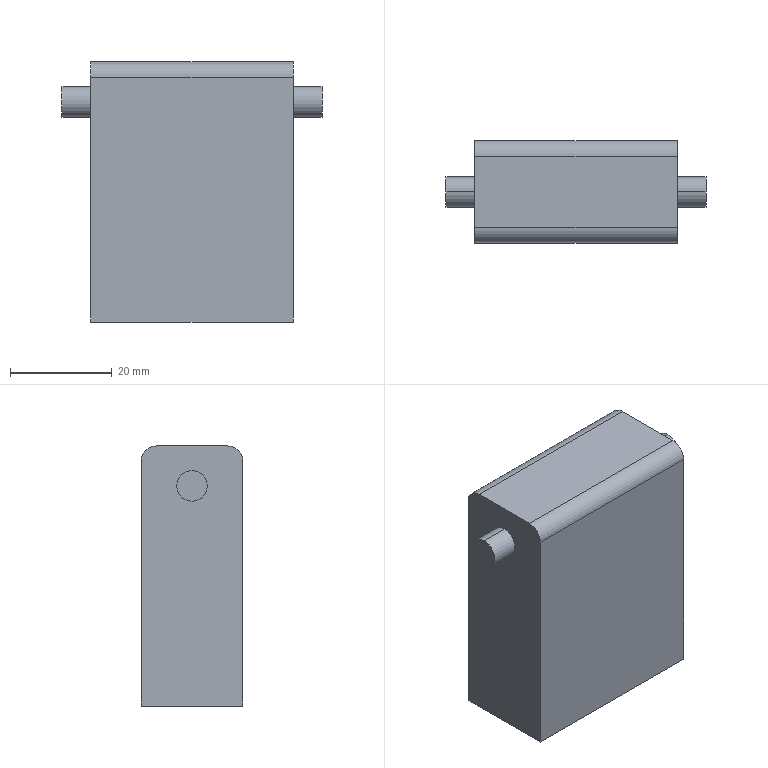Part | SolidWorks | features 3DProfileFeature 1, Extrusion 1, Fillet 1, HoleWzd 1, ICE 1 | 1 solid | 26 faces | box 51 x 20 x 51 mm | volume 40645 mm3 | cylinder 12 | plane 8 | cone 6 | commonest cylinder face diameters 2.5 x6 6 x6
STEP:
#1=CARTESIAN_POINT('',(13.75,0.,7.5));
#2=VERTEX_POINT('',#1);
#3=CARTESIAN_POINT('',(11.25,0.,7.5));
#4=VERTEX_POINT('',#3);
#5=CARTESIAN_POINT('',(12.5,0.,7.5));
#6=DIRECTION('',(0.,0.,-1.));
#7=DIRECTION('',(-1.,0.,0.));
#8=AXIS2_PLACEMENT_3D('',#5,#6,#7);
#9=CIRCLE('',#8,1.25);
#10=EDGE_CURVE('',#2,#4,#9,.T.);
#11=ORIENTED_EDGE('',*,*,#10,.F.);
#12=CARTESIAN_POINT('',(13.75,0.,0.));
#13=VERTEX_POINT('',#12);
#14=CARTESIAN_POINT('',(13.75,0.,0.));
#15=DIRECTION('',(0.,0.,-1.));
#16=VECTOR('',#15,1000.);
#17=LINE('',#14,#16);
#18=EDGE_CURVE('',#2,#13,#17,.T.);
#19=ORIENTED_EDGE('',*,*,#18,.T.);
#20=CARTESIAN_POINT('',(11.25,0.,0.));
#21=VERTEX_POINT('',#20);
#22=CARTESIAN_POINT('',(12.5,0.,0.));
#23=DIRECTION('',(0.,0.,-1.));
#24=DIRECTION('',(-1.,0.,0.));
#25=AXIS2_PLACEMENT_3D('',#22,#23,#24);
#26=CIRCLE('',#25,1.25);
#27=EDGE_CURVE('',#13,#21,#26,.T.);
#28=ORIENTED_EDGE('',*,*,#27,.T.);
#29=CARTESIAN_POINT('',(11.25,0.,0.));
#30=DIRECTION('',(0.,0.,-1.));
#31=VECTOR('',#30,1000.);
#32=LINE('',#29,#31);
#33=EDGE_CURVE('',#4,#21,#32,.T.);
#34=ORIENTED_EDGE('',*,*,#33,.F.);
#35=EDGE_LOOP('',(#11,#19,#28,#34));
#36=FACE_OUTER_BOUND('',#35,.T.);
#37=CARTESIAN_POINT('',(12.5,0.,0.));
#38=DIRECTION('',(0.,0.,-1.));
#39=DIRECTION('',(-1.,0.,0.));
#40=AXIS2_PLACEMENT_3D('',#37,#38,#39);
#41=CYLINDRICAL_SURFACE('',#40,1.25);
#42=ADVANCED_FACE('',(#36),#41,.F.);
#43=CARTESIAN_POINT('',(12.5,0.,8.251));
#44=VERTEX_POINT('',#43);
#45=CARTESIAN_POINT('',(11.25,0.,7.5));
#46=DIRECTION('',(-0.8572,0.,-0.515));
#47=VECTOR('',#46,1000.);
#48=LINE('',#45,#47);
#49=EDGE_CURVE('',#44,#4,#48,.T.);
#50=ORIENTED_EDGE('',*,*,#49,.F.);
#51=CARTESIAN_POINT('',(13.75,0.,7.5));
#52=DIRECTION('',(0.8572,0.,-0.515));
#53=VECTOR('',#52,1000.);
#54=LINE('',#51,#53);
#55=EDGE_CURVE('',#44,#2,#54,.T.);
#56=ORIENTED_EDGE('',*,*,#55,.T.);
#57=ORIENTED_EDGE('',*,*,#10,.T.);
#58=EDGE_LOOP('',(#50,#56,#57));
#59=FACE_OUTER_BOUND('',#58,.T.);
#60=CARTESIAN_POINT('',(12.5,0.,7.5));
#61=DIRECTION('',(0.,0.,-1.));
#62=DIRECTION('',(-1.,0.,0.));
#63=AXIS2_PLACEMENT_3D('',#60,#61,#62);
#64=CONICAL_SURFACE('',#63,1.25,1.03);
#65=ADVANCED_FACE('',(#59),#64,.F.);
#66=CARTESIAN_POINT('',(-11.25,0.,7.5));
#67=VERTEX_POINT('',#66);
#68=CARTESIAN_POINT('',(-13.75,0.,7.5));
#69=VERTEX_POINT('',#68);
#70=CARTESIAN_POINT('',(-12.5,0.,7.5));
#71=DIRECTION('',(0.,0.,-1.));
#72=DIRECTION('',(-1.,0.,0.));
#73=AXIS2_PLACEMENT_3D('',#70,#71,#72);
#74=CIRCLE('',#73,1.25);
#75=EDGE_CURVE('',#67,#69,#74,.T.);
#76=ORIENTED_EDGE('',*,*,#75,.F.);
#77=CARTESIAN_POINT('',(-11.25,0.,0.));
#78=VERTEX_POINT('',#77);
#79=CARTESIAN_POINT('',(-11.25,0.,0.));
#80=DIRECTION('',(0.,0.,-1.));
#81=VECTOR('',#80,1000.);
#82=LINE('',#79,#81);
#83=EDGE_CURVE('',#67,#78,#82,.T.);
#84=ORIENTED_EDGE('',*,*,#83,.T.);
#85=CARTESIAN_POINT('',(-13.75,0.,0.));
#86=VERTEX_POINT('',#85);
#87=CARTESIAN_POINT('',(-12.5,0.,0.));
#88=DIRECTION('',(0.,0.,-1.));
#89=DIRECTION('',(-1.,0.,0.));
#90=AXIS2_PLACEMENT_3D('',#87,#88,#89);
#91=CIRCLE('',#90,1.25);
#92=EDGE_CURVE('',#78,#86,#91,.T.);
#93=ORIENTED_EDGE('',*,*,#92,.T.);
#94=CARTESIAN_POINT('',(-13.75,0.,0.));
#95=DIRECTION('',(0.,0.,-1.));
#96=VECTOR('',#95,1000.);
#97=LINE('',#94,#96);
#98=EDGE_CURVE('',#69,#86,#97,.T.);
#99=ORIENTED_EDGE('',*,*,#98,.F.);
#100=EDGE_LOOP('',(#76,#84,#93,#99));
#101=FACE_OUTER_BOUND('',#100,.T.);
#102=CARTESIAN_POINT('',(-12.5,0.,0.));
#103=DIRECTION('',(0.,0.,-1.));
#104=DIRECTION('',(-1.,0.,0.));
#105=AXIS2_PLACEMENT_3D('',#102,#103,#104);
#106=CYLINDRICAL_SURFACE('',#105,1.25);
#107=ADVANCED_FACE('',(#101),#106,.F.);
#108=CARTESIAN_POINT('',(-12.5,0.,8.251));
#109=VERTEX_POINT('',#108);
#110=CARTESIAN_POINT('',(-13.75,0.,7.5));
#111=DIRECTION('',(-0.8572,0.,-0.515));
#112=VECTOR('',#111,1000.);
#113=LINE('',#110,#112);
#114=EDGE_CURVE('',#109,#69,#113,.T.);
#115=ORIENTED_EDGE('',*,*,#114,.F.);
#116=CARTESIAN_POINT('',(-11.25,0.,7.5));
#117=DIRECTION('',(0.8572,0.,-0.515));
#118=VECTOR('',#117,1000.);
#119=LINE('',#116,#118);
#120=EDGE_CURVE('',#109,#67,#119,.T.);
#121=ORIENTED_EDGE('',*,*,#120,.T.);
#122=ORIENTED_EDGE('',*,*,#75,.T.);
#123=EDGE_LOOP('',(#115,#121,#122));
#124=FACE_OUTER_BOUND('',#123,.T.);
#125=CARTESIAN_POINT('',(-12.5,0.,7.5));
#126=DIRECTION('',(0.,0.,-1.));
#127=DIRECTION('',(-1.,0.,0.));
#128=AXIS2_PLACEMENT_3D('',#125,#126,#127);
#129=CONICAL_SURFACE('',#128,1.25,1.03);
#130=ADVANCED_FACE('',(#124),#129,.F.);
#131=CARTESIAN_POINT('',(1.129,0.,7.5));
#132=VERTEX_POINT('',#131);
#133=CARTESIAN_POINT('',(-1.371,0.,7.5));
#134=VERTEX_POINT('',#133);
#135=CARTESIAN_POINT('',(-0.1209,0.,7.5));
#136=DIRECTION('',(0.,0.,-1.));
#137=DIRECTION('',(-1.,0.,0.));
#138=AXIS2_PLACEMENT_3D('',#135,#136,#137);
#139=CIRCLE('',#138,1.25);
#140=EDGE_CURVE('',#132,#134,#139,.T.);
#141=ORIENTED_EDGE('',*,*,#140,.F.);
#142=CARTESIAN_POINT('',(1.129,0.,0.));
#143=VERTEX_POINT('',#142);
#144=CARTESIAN_POINT('',(1.129,0.,0.));
#145=DIRECTION('',(0.,0.,-1.));
#146=VECTOR('',#145,1000.);
#147=LINE('',#144,#146);
#148=EDGE_CURVE('',#132,#143,#147,.T.);
#149=ORIENTED_EDGE('',*,*,#148,.T.);
#150=CARTESIAN_POINT('',(-1.371,0.,0.));
#151=VERTEX_POINT('',#150);
#152=CARTESIAN_POINT('',(-0.1209,0.,0.));
#153=DIRECTION('',(0.,0.,-1.));
#154=DIRECTION('',(-1.,0.,0.));
#155=AXIS2_PLACEMENT_3D('',#152,#153,#154);
#156=CIRCLE('',#155,1.25);
#157=EDGE_CURVE('',#143,#151,#156,.T.);
#158=ORIENTED_EDGE('',*,*,#157,.T.);
#159=CARTESIAN_POINT('',(-1.371,0.,0.));
#160=DIRECTION('',(0.,0.,-1.));
#161=VECTOR('',#160,1000.);
#162=LINE('',#159,#161);
#163=EDGE_CURVE('',#134,#151,#162,.T.);
#164=ORIENTED_EDGE('',*,*,#163,.F.);
#165=EDGE_LOOP('',(#141,#149,#158,#164));
#166=FACE_OUTER_BOUND('',#165,.T.);
#167=CARTESIAN_POINT('',(-0.1209,0.,0.));
#168=DIRECTION('',(0.,0.,-1.));
#169=DIRECTION('',(-1.,0.,0.));
#170=AXIS2_PLACEMENT_3D('',#167,#168,#169);
#171=CYLINDRICAL_SURFACE('',#170,1.25);
#172=ADVANCED_FACE('',(#166),#171,.F.);
#173=CARTESIAN_POINT('',(-0.1209,0.,8.251));
#174=VERTEX_POINT('',#173);
#175=CARTESIAN_POINT('',(-1.371,0.,7.5));
#176=DIRECTION('',(-0.8572,0.,-0.515));
#177=VECTOR('',#176,1000.);
#178=LINE('',#175,#177);
#179=EDGE_CURVE('',#174,#134,#178,.T.);
#180=ORIENTED_EDGE('',*,*,#179,.F.);
#181=CARTESIAN_POINT('',(1.129,0.,7.5));
#182=DIRECTION('',(0.8572,0.,-0.515));
#183=VECTOR('',#182,1000.);
#184=LINE('',#181,#183);
#185=EDGE_CURVE('',#174,#132,#184,.T.);
#186=ORIENTED_EDGE('',*,*,#185,.T.);
#187=ORIENTED_EDGE('',*,*,#140,.T.);
#188=EDGE_LOOP('',(#180,#186,#187));
#189=FACE_OUTER_BOUND('',#188,.T.);
#190=CARTESIAN_POINT('',(-0.1209,0.,7.5));
#191=DIRECTION('',(0.,0.,-1.));
#192=DIRECTION('',(-1.,0.,0.));
#193=AXIS2_PLACEMENT_3D('',#190,#191,#192);
#194=CONICAL_SURFACE('',#193,1.25,1.03);
#195=ADVANCED_FACE('',(#189),#194,.F.);
#196=CARTESIAN_POINT('',(25.5,0.,40.174));
#197=VERTEX_POINT('',#196);
#198=CARTESIAN_POINT('',(25.5,0.,46.174));
#199=VERTEX_POINT('',#198);
#200=CARTESIAN_POINT('',(25.5,0.,43.174));
#201=DIRECTION('',(1.,0.,0.));
#202=DIRECTION('',(0.,0.,-1.));
#203=AXIS2_PLACEMENT_3D('',#200,#201,#202);
#204=CIRCLE('',#203,3.);
#205=EDGE_CURVE('',#197,#199,#204,.T.);
#206=ORIENTED_EDGE('',*,*,#205,.F.);
#207=CARTESIAN_POINT('',(19.9,0.,40.174));
#208=VERTEX_POINT('',#207);
#209=CARTESIAN_POINT('',(25.5,0.,40.174));
#210=DIRECTION('',(-1.,0.,0.));
#211=VECTOR('',#210,1000.);
#212=LINE('',#209,#211);
#213=EDGE_CURVE('',#197,#208,#212,.T.);
#214=ORIENTED_EDGE('',*,*,#213,.T.);
#215=CARTESIAN_POINT('',(19.9,0.,46.174));
#216=VERTEX_POINT('',#215);
#217=CARTESIAN_POINT('',(19.9,0.,43.174));
#218=DIRECTION('',(1.,0.,0.));
#219=DIRECTION('',(0.,-1.,0.));
#220=AXIS2_PLACEMENT_3D('',#217,#218,#219);
#221=CIRCLE('',#220,3.);
#222=EDGE_CURVE('',#208,#216,#221,.T.);
#223=ORIENTED_EDGE('',*,*,#222,.T.);
#224=CARTESIAN_POINT('',(25.5,0.,46.174));
#225=DIRECTION('',(-1.,0.,0.));
#226=VECTOR('',#225,1000.);
#227=LINE('',#224,#226);
#228=EDGE_CURVE('',#199,#216,#227,.T.);
#229=ORIENTED_EDGE('',*,*,#228,.F.);
#230=EDGE_LOOP('',(#206,#214,#223,#229));
#231=FACE_OUTER_BOUND('',#230,.T.);
#232=CARTESIAN_POINT('',(25.5,0.,43.174));
#233=DIRECTION('',(-1.,0.,0.));
#234=DIRECTION('',(0.,0.,1.));
#235=AXIS2_PLACEMENT_3D('',#232,#233,#234);
#236=CYLINDRICAL_SURFACE('',#235,3.);
#237=ADVANCED_FACE('',(#231),#236,.T.);
#238=CARTESIAN_POINT('',(-19.9,0.,46.174));
#239=VERTEX_POINT('',#238);
#240=CARTESIAN_POINT('',(-19.9,0.,40.174));
#241=VERTEX_POINT('',#240);
#242=CARTESIAN_POINT('',(-19.9,0.,43.174));
#243=DIRECTION('',(-1.,0.,0.));
#244=DIRECTION('',(0.,1.,0.));
#245=AXIS2_PLACEMENT_3D('',#242,#243,#244);
#246=CIRCLE('',#245,3.);
#247=EDGE_CURVE('',#239,#241,#246,.T.);
#248=ORIENTED_EDGE('',*,*,#247,.T.);
#249=CARTESIAN_POINT('',(-25.5,0.,40.174));
#250=VERTEX_POINT('',#249);
#251=CARTESIAN_POINT('',(25.5,0.,40.174));
#252=DIRECTION('',(-1.,0.,0.));
#253=VECTOR('',#252,1000.);
#254=LINE('',#251,#253);
#255=EDGE_CURVE('',#241,#250,#254,.T.);
#256=ORIENTED_EDGE('',*,*,#255,.T.);
#257=CARTESIAN_POINT('',(-25.5,0.,46.174));
#258=VERTEX_POINT('',#257);
#259=CARTESIAN_POINT('',(-25.5,0.,43.174));
#260=DIRECTION('',(1.,0.,0.));
#261=DIRECTION('',(0.,0.,-1.));
#262=AXIS2_PLACEMENT_3D('',#259,#260,#261);
#263=CIRCLE('',#262,3.);
#264=EDGE_CURVE('',#250,#258,#263,.T.);
#265=ORIENTED_EDGE('',*,*,#264,.T.);
#266=CARTESIAN_POINT('',(25.5,0.,46.174));
#267=DIRECTION('',(-1.,0.,0.));
#268=VECTOR('',#267,1000.);
#269=LINE('',#266,#268);
#270=EDGE_CURVE('',#239,#258,#269,.T.);
#271=ORIENTED_EDGE('',*,*,#270,.F.);
#272=EDGE_LOOP('',(#248,#256,#265,#271));
#273=FACE_OUTER_BOUND('',#272,.T.);
#274=CARTESIAN_POINT('',(25.5,0.,43.174));
#275=DIRECTION('',(-1.,0.,0.));
#276=DIRECTION('',(0.,0.,1.));
#277=AXIS2_PLACEMENT_3D('',#274,#275,#276);
#278=CYLINDRICAL_SURFACE('',#277,3.);
#279=ADVANCED_FACE('',(#273),#278,.T.);
#280=CARTESIAN_POINT('',(19.9,0.,43.174));
#281=DIRECTION('',(1.,0.,0.));
#282=DIRECTION('',(0.,-1.,0.));
#283=AXIS2_PLACEMENT_3D('',#280,#281,#282);
#284=CIRCLE('',#283,3.);
#285=EDGE_CURVE('',#216,#208,#284,.T.);
#286=ORIENTED_EDGE('',*,*,#285,.F.);
#287=ORIENTED_EDGE('',*,*,#222,.F.);
#288=EDGE_LOOP('',(#286,#287));
#289=FACE_BOUND('',#288,.T.);
#290=CARTESIAN_POINT('',(19.9,-7.,51.));
#291=VERTEX_POINT('',#290);
#292=CARTESIAN_POINT('',(19.9,7.,51.));
#293=VERTEX_POINT('',#292);
#294=CARTESIAN_POINT('',(19.9,10.,51.));
#295=DIRECTION('',(0.,1.,0.));
#296=VECTOR('',#295,1000.);
#297=LINE('',#294,#296);
#298=EDGE_CURVE('',#291,#293,#297,.T.);
#299=ORIENTED_EDGE('',*,*,#298,.F.);
#300=CARTESIAN_POINT('',(19.9,-10.,48.));
#301=VERTEX_POINT('',#300);
#302=CARTESIAN_POINT('',(19.9,-7.,48.));
#303=DIRECTION('',(1.,0.,0.));
#304=DIRECTION('',(0.,-1.,0.));
#305=AXIS2_PLACEMENT_3D('',#302,#303,#304);
#306=CIRCLE('',#305,3.);
#307=EDGE_CURVE('',#291,#301,#306,.T.);
#308=ORIENTED_EDGE('',*,*,#307,.T.);
#309=CARTESIAN_POINT('',(19.9,-10.,0.));
#310=VERTEX_POINT('',#309);
#311=CARTESIAN_POINT('',(19.9,-10.,51.));
#312=DIRECTION('',(0.,0.,-1.));
#313=VECTOR('',#312,1000.);
#314=LINE('',#311,#313);
#315=EDGE_CURVE('',#301,#310,#314,.T.);
#316=ORIENTED_EDGE('',*,*,#315,.T.);
#317=CARTESIAN_POINT('',(19.9,10.,0.));
#318=VERTEX_POINT('',#317);
#319=CARTESIAN_POINT('',(19.9,10.,0.));
#320=DIRECTION('',(0.,1.,0.));
#321=VECTOR('',#320,1000.);
#322=LINE('',#319,#321);
#323=EDGE_CURVE('',#310,#318,#322,.T.);
#324=ORIENTED_EDGE('',*,*,#323,.T.);
#325=CARTESIAN_POINT('',(19.9,10.,48.));
#326=VERTEX_POINT('',#325);
#327=CARTESIAN_POINT('',(19.9,10.,51.));
#328=DIRECTION('',(0.,0.,-1.));
#329=VECTOR('',#328,1000.);
#330=LINE('',#327,#329);
#331=EDGE_CURVE('',#326,#318,#330,.T.);
#332=ORIENTED_EDGE('',*,*,#331,.F.);
#333=CARTESIAN_POINT('',(19.9,7.,48.));
#334=DIRECTION('',(1.,0.,0.));
#335=DIRECTION('',(0.,-1.,0.));
#336=AXIS2_PLACEMENT_3D('',#333,#334,#335);
#337=CIRCLE('',#336,3.);
#338=EDGE_CURVE('',#326,#293,#337,.T.);
#339=ORIENTED_EDGE('',*,*,#338,.T.);
#340=EDGE_LOOP('',(#299,#308,#316,#324,#332,#339));
#341=FACE_OUTER_BOUND('',#340,.T.);
#342=CARTESIAN_POINT('',(19.9,10.,51.));
#343=DIRECTION('',(-1.,0.,0.));
#344=DIRECTION('',(0.,-1.,0.));
#345=AXIS2_PLACEMENT_3D('',#342,#343,#344);
#346=PLANE('',#345);
#347=ADVANCED_FACE('',(#289,#341),#346,.F.);
#348=CARTESIAN_POINT('',(-19.9,10.,48.));
#349=VERTEX_POINT('',#348);
#350=CARTESIAN_POINT('',(-19.9,10.,0.));
#351=VERTEX_POINT('',#350);
#352=CARTESIAN_POINT('',(-19.9,10.,51.));
#353=DIRECTION('',(0.,0.,-1.));
#354=VECTOR('',#353,1000.);
#355=LINE('',#352,#354);
#356=EDGE_CURVE('',#349,#351,#355,.T.);
#357=ORIENTED_EDGE('',*,*,#356,.F.);
#358=CARTESIAN_POINT('',(19.9,10.,48.));
#359=DIRECTION('',(1.,0.,0.));
#360=VECTOR('',#359,1000.);
#361=LINE('',#358,#360);
#362=EDGE_CURVE('',#349,#326,#361,.T.);
#363=ORIENTED_EDGE('',*,*,#362,.T.);
#364=ORIENTED_EDGE('',*,*,#331,.T.);
#365=CARTESIAN_POINT('',(-19.9,10.,0.));
#366=DIRECTION('',(-1.,0.,0.));
#367=VECTOR('',#366,1000.);
#368=LINE('',#365,#367);
#369=EDGE_CURVE('',#318,#351,#368,.T.);
#370=ORIENTED_EDGE('',*,*,#369,.T.);
#371=EDGE_LOOP('',(#357,#363,#364,#370));
#372=FACE_OUTER_BOUND('',#371,.T.);
#373=CARTESIAN_POINT('',(-19.9,10.,51.));
#374=DIRECTION('',(0.,-1.,0.));
#375=DIRECTION('',(0.,0.,-1.));
#376=AXIS2_PLACEMENT_3D('',#373,#374,#375);
#377=PLANE('',#376);
#378=ADVANCED_FACE('',(#372),#377,.F.);
#379=ORIENTED_EDGE('',*,*,#247,.F.);
#380=CARTESIAN_POINT('',(-19.9,0.,43.174));
#381=DIRECTION('',(-1.,0.,0.));
#382=DIRECTION('',(0.,1.,0.));
#383=AXIS2_PLACEMENT_3D('',#380,#381,#382);
#384=CIRCLE('',#383,3.);
#385=EDGE_CURVE('',#241,#239,#384,.T.);
#386=ORIENTED_EDGE('',*,*,#385,.F.);
#387=EDGE_LOOP('',(#379,#386));
#388=FACE_BOUND('',#387,.T.);
#389=CARTESIAN_POINT('',(-19.9,-10.,48.));
#390=VERTEX_POINT('',#389);
#391=CARTESIAN_POINT('',(-19.9,-10.,0.));
#392=VERTEX_POINT('',#391);
#393=CARTESIAN_POINT('',(-19.9,-10.,51.));
#394=DIRECTION('',(0.,0.,-1.));
#395=VECTOR('',#394,1000.);
#396=LINE('',#393,#395);
#397=EDGE_CURVE('',#390,#392,#396,.T.);
#398=ORIENTED_EDGE('',*,*,#397,.F.);
#399=CARTESIAN_POINT('',(-19.9,-7.,51.));
#400=VERTEX_POINT('',#399);
#401=CARTESIAN_POINT('',(-19.9,-7.,48.));
#402=DIRECTION('',(-1.,0.,0.));
#403=DIRECTION('',(0.,1.,0.));
#404=AXIS2_PLACEMENT_3D('',#401,#402,#403);
#405=CIRCLE('',#404,3.);
#406=EDGE_CURVE('',#390,#400,#405,.T.);
#407=ORIENTED_EDGE('',*,*,#406,.T.);
#408=CARTESIAN_POINT('',(-19.9,7.,51.));
#409=VERTEX_POINT('',#408);
#410=CARTESIAN_POINT('',(-19.9,10.,51.));
#411=DIRECTION('',(0.,-1.,0.));
#412=VECTOR('',#411,1000.);
#413=LINE('',#410,#412);
#414=EDGE_CURVE('',#409,#400,#413,.T.);
#415=ORIENTED_EDGE('',*,*,#414,.F.);
#416=CARTESIAN_POINT('',(-19.9,7.,48.));
#417=DIRECTION('',(-1.,0.,0.));
#418=DIRECTION('',(0.,1.,0.));
#419=AXIS2_PLACEMENT_3D('',#416,#417,#418);
#420=CIRCLE('',#419,3.);
#421=EDGE_CURVE('',#409,#349,#420,.T.);
#422=ORIENTED_EDGE('',*,*,#421,.T.);
#423=ORIENTED_EDGE('',*,*,#356,.T.);
#424=CARTESIAN_POINT('',(-19.9,10.,0.));
#425=DIRECTION('',(0.,-1.,0.));
#426=VECTOR('',#425,1000.);
#427=LINE('',#424,#426);
#428=EDGE_CURVE('',#351,#392,#427,.T.);
#429=ORIENTED_EDGE('',*,*,#428,.T.);
#430=EDGE_LOOP('',(#398,#407,#415,#422,#423,#429));
#431=FACE_OUTER_BOUND('',#430,.T.);
#432=CARTESIAN_POINT('',(-19.9,10.,51.));
#433=DIRECTION('',(1.,0.,0.));
#434=DIRECTION('',(0.,1.,0.));
#435=AXIS2_PLACEMENT_3D('',#432,#433,#434);
#436=PLANE('',#435);
#437=ADVANCED_FACE('',(#388,#431),#436,.F.);
#438=ORIENTED_EDGE('',*,*,#315,.F.);
#439=CARTESIAN_POINT('',(-19.9,-10.,48.));
#440=DIRECTION('',(-1.,0.,0.));
#441=VECTOR('',#440,1000.);
#442=LINE('',#439,#441);
#443=EDGE_CURVE('',#301,#390,#442,.T.);
#444=ORIENTED_EDGE('',*,*,#443,.T.);
#445=ORIENTED_EDGE('',*,*,#397,.T.);
#446=CARTESIAN_POINT('',(-19.9,-10.,0.));
#447=DIRECTION('',(1.,0.,0.));
#448=VECTOR('',#447,1000.);
#449=LINE('',#446,#448);
#450=EDGE_CURVE('',#392,#310,#449,.T.);
#451=ORIENTED_EDGE('',*,*,#450,.T.);
#452=EDGE_LOOP('',(#438,#444,#445,#451));
#453=FACE_OUTER_BOUND('',#452,.T.);
#454=CARTESIAN_POINT('',(-19.9,-10.,51.));
#455=DIRECTION('',(0.,1.,0.));
#456=DIRECTION('',(0.,0.,1.));
#457=AXIS2_PLACEMENT_3D('',#454,#455,#456);
#458=PLANE('',#457);
#459=ADVANCED_FACE('',(#453),#458,.F.);
#460=ORIENTED_EDGE('',*,*,#414,.T.);
#461=CARTESIAN_POINT('',(19.9,-7.,51.));
#462=DIRECTION('',(1.,0.,0.));
#463=VECTOR('',#462,1000.);
#464=LINE('',#461,#463);
#465=EDGE_CURVE('',#400,#291,#464,.T.);
#466=ORIENTED_EDGE('',*,*,#465,.T.);
#467=ORIENTED_EDGE('',*,*,#298,.T.);
#468=CARTESIAN_POINT('',(-19.9,7.,51.));
#469=DIRECTION('',(-1.,0.,0.));
#470=VECTOR('',#469,1000.);
#471=LINE('',#468,#470);
#472=EDGE_CURVE('',#293,#409,#471,.T.);
#473=ORIENTED_EDGE('',*,*,#472,.T.);
#474=EDGE_LOOP('',(#460,#466,#467,#473));
#475=FACE_OUTER_BOUND('',#474,.T.);
#476=CARTESIAN_POINT('',(0.,0.,51.));
#477=DIRECTION('',(0.,0.,1.));
#478=DIRECTION('',(1.,0.,0.));
#479=AXIS2_PLACEMENT_3D('',#476,#477,#478);
#480=PLANE('',#479);
#481=ADVANCED_FACE('',(#475),#480,.T.);
#482=CARTESIAN_POINT('',(12.5,0.,0.));
#483=DIRECTION('',(0.,0.,-1.));
#484=DIRECTION('',(-1.,0.,0.));
#485=AXIS2_PLACEMENT_3D('',#482,#483,#484);
#486=CIRCLE('',#485,1.25);
#487=EDGE_CURVE('',#21,#13,#486,.T.);
#488=ORIENTED_EDGE('',*,*,#487,.F.);
#489=ORIENTED_EDGE('',*,*,#27,.F.);
#490=EDGE_LOOP('',(#488,#489));
#491=FACE_BOUND('',#490,.T.);
#492=CARTESIAN_POINT('',(-12.5,0.,0.));
#493=DIRECTION('',(0.,0.,-1.));
#494=DIRECTION('',(-1.,0.,0.));
#495=AXIS2_PLACEMENT_3D('',#492,#493,#494);
#496=CIRCLE('',#495,1.25);
#497=EDGE_CURVE('',#86,#78,#496,.T.);
#498=ORIENTED_EDGE('',*,*,#497,.F.);
#499=ORIENTED_EDGE('',*,*,#92,.F.);
#500=EDGE_LOOP('',(#498,#499));
#501=FACE_BOUND('',#500,.T.);
#502=CARTESIAN_POINT('',(-0.1209,0.,0.));
#503=DIRECTION('',(0.,0.,-1.));
#504=DIRECTION('',(-1.,0.,0.));
#505=AXIS2_PLACEMENT_3D('',#502,#503,#504);
#506=CIRCLE('',#505,1.25);
#507=EDGE_CURVE('',#151,#143,#506,.T.);
#508=ORIENTED_EDGE('',*,*,#507,.F.);
#509=ORIENTED_EDGE('',*,*,#157,.F.);
#510=EDGE_LOOP('',(#508,#509));
#511=FACE_BOUND('',#510,.T.);
#512=ORIENTED_EDGE('',*,*,#323,.F.);
#513=ORIENTED_EDGE('',*,*,#450,.F.);
#514=ORIENTED_EDGE('',*,*,#428,.F.);
#515=ORIENTED_EDGE('',*,*,#369,.F.);
#516=EDGE_LOOP('',(#512,#513,#514,#515));
#517=FACE_OUTER_BOUND('',#516,.T.);
#518=CARTESIAN_POINT('',(0.,0.,0.));
#519=DIRECTION('',(0.,0.,1.));
#520=DIRECTION('',(1.,0.,0.));
#521=AXIS2_PLACEMENT_3D('',#518,#519,#520);
#522=PLANE('',#521);
#523=ADVANCED_FACE('',(#491,#501,#511,#517),#522,.F.);
#524=CARTESIAN_POINT('',(-25.5,0.,43.174));
#525=DIRECTION('',(1.,0.,0.));
#526=DIRECTION('',(0.,0.,-1.));
#527=AXIS2_PLACEMENT_3D('',#524,#525,#526);
#528=CIRCLE('',#527,3.);
#529=EDGE_CURVE('',#258,#250,#528,.T.);
#530=ORIENTED_EDGE('',*,*,#529,.F.);
#531=ORIENTED_EDGE('',*,*,#264,.F.);
#532=EDGE_LOOP('',(#530,#531));
#533=FACE_OUTER_BOUND('',#532,.T.);
#534=CARTESIAN_POINT('',(-25.5,0.,43.174));
#535=DIRECTION('',(1.,0.,0.));
#536=DIRECTION('',(0.,0.,-1.));
#537=AXIS2_PLACEMENT_3D('',#534,#535,#536);
#538=PLANE('',#537);
#539=ADVANCED_FACE('',(#533),#538,.F.);
#540=ORIENTED_EDGE('',*,*,#255,.F.);
#541=ORIENTED_EDGE('',*,*,#385,.T.);
#542=ORIENTED_EDGE('',*,*,#270,.T.);
#543=ORIENTED_EDGE('',*,*,#529,.T.);
#544=EDGE_LOOP('',(#540,#541,#542,#543));
#545=FACE_OUTER_BOUND('',#544,.T.);
#546=CARTESIAN_POINT('',(25.5,0.,43.174));
#547=DIRECTION('',(-1.,0.,0.));
#548=DIRECTION('',(0.,0.,1.));
#549=AXIS2_PLACEMENT_3D('',#546,#547,#548);
#550=CYLINDRICAL_SURFACE('',#549,3.);
#551=ADVANCED_FACE('',(#545),#550,.T.);
#552=ORIENTED_EDGE('',*,*,#213,.F.);
#553=CARTESIAN_POINT('',(25.5,0.,43.174));
#554=DIRECTION('',(1.,0.,0.));
#555=DIRECTION('',(0.,0.,-1.));
#556=AXIS2_PLACEMENT_3D('',#553,#554,#555);
#557=CIRCLE('',#556,3.);
#558=EDGE_CURVE('',#199,#197,#557,.T.);
#559=ORIENTED_EDGE('',*,*,#558,.F.);
#560=ORIENTED_EDGE('',*,*,#228,.T.);
#561=ORIENTED_EDGE('',*,*,#285,.T.);
#562=EDGE_LOOP('',(#552,#559,#560,#561));
#563=FACE_OUTER_BOUND('',#562,.T.);
#564=CARTESIAN_POINT('',(25.5,0.,43.174));
#565=DIRECTION('',(-1.,0.,0.));
#566=DIRECTION('',(0.,0.,1.));
#567=AXIS2_PLACEMENT_3D('',#564,#565,#566);
#568=CYLINDRICAL_SURFACE('',#567,3.);
#569=ADVANCED_FACE('',(#563),#568,.T.);
#570=ORIENTED_EDGE('',*,*,#558,.T.);
#571=ORIENTED_EDGE('',*,*,#205,.T.);
#572=EDGE_LOOP('',(#570,#571));
#573=FACE_OUTER_BOUND('',#572,.T.);
#574=CARTESIAN_POINT('',(25.5,0.,43.174));
#575=DIRECTION('',(1.,0.,0.));
#576=DIRECTION('',(0.,0.,-1.));
#577=AXIS2_PLACEMENT_3D('',#574,#575,#576);
#578=PLANE('',#577);
#579=ADVANCED_FACE('',(#573),#578,.T.);
#580=ORIENTED_EDGE('',*,*,#185,.F.);
#581=ORIENTED_EDGE('',*,*,#179,.T.);
#582=CARTESIAN_POINT('',(-0.1209,0.,7.5));
#583=DIRECTION('',(0.,0.,-1.));
#584=DIRECTION('',(-1.,0.,0.));
#585=AXIS2_PLACEMENT_3D('',#582,#583,#584);
#586=CIRCLE('',#585,1.25);
#587=EDGE_CURVE('',#134,#132,#586,.T.);
#588=ORIENTED_EDGE('',*,*,#587,.T.);
#589=EDGE_LOOP('',(#580,#581,#588));
#590=FACE_OUTER_BOUND('',#589,.T.);
#591=CARTESIAN_POINT('',(-0.1209,0.,7.5));
#592=DIRECTION('',(0.,0.,-1.));
#593=DIRECTION('',(-1.,0.,0.));
#594=AXIS2_PLACEMENT_3D('',#591,#592,#593);
#595=CONICAL_SURFACE('',#594,1.25,1.03);
#596=ADVANCED_FACE('',(#590),#595,.F.);
#597=ORIENTED_EDGE('',*,*,#148,.F.);
#598=ORIENTED_EDGE('',*,*,#587,.F.);
#599=ORIENTED_EDGE('',*,*,#163,.T.);
#600=ORIENTED_EDGE('',*,*,#507,.T.);
#601=EDGE_LOOP('',(#597,#598,#599,#600));
#602=FACE_OUTER_BOUND('',#601,.T.);
#603=CARTESIAN_POINT('',(-0.1209,0.,0.));
#604=DIRECTION('',(0.,0.,-1.));
#605=DIRECTION('',(-1.,0.,0.));
#606=AXIS2_PLACEMENT_3D('',#603,#604,#605);
#607=CYLINDRICAL_SURFACE('',#606,1.25);
#608=ADVANCED_FACE('',(#602),#607,.F.);
#609=ORIENTED_EDGE('',*,*,#120,.F.);
#610=ORIENTED_EDGE('',*,*,#114,.T.);
#611=CARTESIAN_POINT('',(-12.5,0.,7.5));
#612=DIRECTION('',(0.,0.,-1.));
#613=DIRECTION('',(-1.,0.,0.));
#614=AXIS2_PLACEMENT_3D('',#611,#612,#613);
#615=CIRCLE('',#614,1.25);
#616=EDGE_CURVE('',#69,#67,#615,.T.);
#617=ORIENTED_EDGE('',*,*,#616,.T.);
#618=EDGE_LOOP('',(#609,#610,#617));
#619=FACE_OUTER_BOUND('',#618,.T.);
#620=CARTESIAN_POINT('',(-12.5,0.,7.5));
#621=DIRECTION('',(0.,0.,-1.));
#622=DIRECTION('',(-1.,0.,0.));
#623=AXIS2_PLACEMENT_3D('',#620,#621,#622);
#624=CONICAL_SURFACE('',#623,1.25,1.03);
#625=ADVANCED_FACE('',(#619),#624,.F.);
#626=ORIENTED_EDGE('',*,*,#83,.F.);
#627=ORIENTED_EDGE('',*,*,#616,.F.);
#628=ORIENTED_EDGE('',*,*,#98,.T.);
#629=ORIENTED_EDGE('',*,*,#497,.T.);
#630=EDGE_LOOP('',(#626,#627,#628,#629));
#631=FACE_OUTER_BOUND('',#630,.T.);
#632=CARTESIAN_POINT('',(-12.5,0.,0.));
#633=DIRECTION('',(0.,0.,-1.));
#634=DIRECTION('',(-1.,0.,0.));
#635=AXIS2_PLACEMENT_3D('',#632,#633,#634);
#636=CYLINDRICAL_SURFACE('',#635,1.25);
#637=ADVANCED_FACE('',(#631),#636,.F.);
#638=ORIENTED_EDGE('',*,*,#55,.F.);
#639=ORIENTED_EDGE('',*,*,#49,.T.);
#640=CARTESIAN_POINT('',(12.5,0.,7.5));
#641=DIRECTION('',(0.,0.,-1.));
#642=DIRECTION('',(-1.,0.,0.));
#643=AXIS2_PLACEMENT_3D('',#640,#641,#642);
#644=CIRCLE('',#643,1.25);
#645=EDGE_CURVE('',#4,#2,#644,.T.);
#646=ORIENTED_EDGE('',*,*,#645,.T.);
#647=EDGE_LOOP('',(#638,#639,#646));
#648=FACE_OUTER_BOUND('',#647,.T.);
#649=CARTESIAN_POINT('',(12.5,0.,7.5));
#650=DIRECTION('',(0.,0.,-1.));
#651=DIRECTION('',(-1.,0.,0.));
#652=AXIS2_PLACEMENT_3D('',#649,#650,#651);
#653=CONICAL_SURFACE('',#652,1.25,1.03);
#654=ADVANCED_FACE('',(#648),#653,.F.);
#655=ORIENTED_EDGE('',*,*,#18,.F.);
#656=ORIENTED_EDGE('',*,*,#645,.F.);
#657=ORIENTED_EDGE('',*,*,#33,.T.);
#658=ORIENTED_EDGE('',*,*,#487,.T.);
#659=EDGE_LOOP('',(#655,#656,#657,#658));
#660=FACE_OUTER_BOUND('',#659,.T.);
#661=CARTESIAN_POINT('',(12.5,0.,0.));
#662=DIRECTION('',(0.,0.,-1.));
#663=DIRECTION('',(-1.,0.,0.));
#664=AXIS2_PLACEMENT_3D('',#661,#662,#663);
#665=CYLINDRICAL_SURFACE('',#664,1.25);
#666=ADVANCED_FACE('',(#660),#665,.F.);
#667=ORIENTED_EDGE('',*,*,#406,.F.);
#668=ORIENTED_EDGE('',*,*,#443,.F.);
#669=ORIENTED_EDGE('',*,*,#307,.F.);
#670=ORIENTED_EDGE('',*,*,#465,.F.);
#671=EDGE_LOOP('',(#667,#668,#669,#670));
#672=FACE_OUTER_BOUND('',#671,.T.);
#673=CARTESIAN_POINT('',(0.,-7.,48.));
#674=DIRECTION('',(-1.,0.,0.));
#675=DIRECTION('',(0.,0.,1.));
#676=AXIS2_PLACEMENT_3D('',#673,#674,#675);
#677=CYLINDRICAL_SURFACE('',#676,3.);
#678=ADVANCED_FACE('',(#672),#677,.T.);
#679=ORIENTED_EDGE('',*,*,#338,.F.);
#680=ORIENTED_EDGE('',*,*,#362,.F.);
#681=ORIENTED_EDGE('',*,*,#421,.F.);
#682=ORIENTED_EDGE('',*,*,#472,.F.);
#683=EDGE_LOOP('',(#679,#680,#681,#682));
#684=FACE_OUTER_BOUND('',#683,.T.);
#685=CARTESIAN_POINT('',(0.,7.,48.));
#686=DIRECTION('',(1.,0.,0.));
#687=DIRECTION('',(0.,0.,-1.));
#688=AXIS2_PLACEMENT_3D('',#685,#686,#687);
#689=CYLINDRICAL_SURFACE('',#688,3.);
#690=ADVANCED_FACE('',(#684),#689,.T.);
#691=CLOSED_SHELL('',(#42,#65,#107,#130,#172,#195,#237,#279,#347,#378,#437,#459,#481,#523,#539,#551,#569,#579,#596,#608,#625,#637,#654,#666,#678,#690));
#692=MANIFOLD_SOLID_BREP('',#691);
#693=CARTESIAN_POINT('',(0.,0.,0.));
#694=DIRECTION('',(0.,0.,1.));
#695=DIRECTION('',(1.,0.,0.));
#696=AXIS2_PLACEMENT_3D('',#693,#694,#695);
#697=(LENGTH_UNIT()NAMED_UNIT(*)SI_UNIT(.MILLI.,.METRE.));
#698=UNCERTAINTY_MEASURE_WITH_UNIT(LENGTH_MEASURE(0.00001),#697,'','');
#699=(NAMED_UNIT(*)PLANE_ANGLE_UNIT()SI_UNIT($,.RADIAN.));
#700=(NAMED_UNIT(*)SI_UNIT($,.STERADIAN.)SOLID_ANGLE_UNIT());
#701=(GEOMETRIC_REPRESENTATION_CONTEXT(3)GLOBAL_UNCERTAINTY_ASSIGNED_CONTEXT((#698))GLOBAL_UNIT_ASSIGNED_CONTEXT((#697,#699,#700))REPRESENTATION_CONTEXT('',''));
#702=ADVANCED_BREP_SHAPE_REPRESENTATION('',(#692,#696),#701);